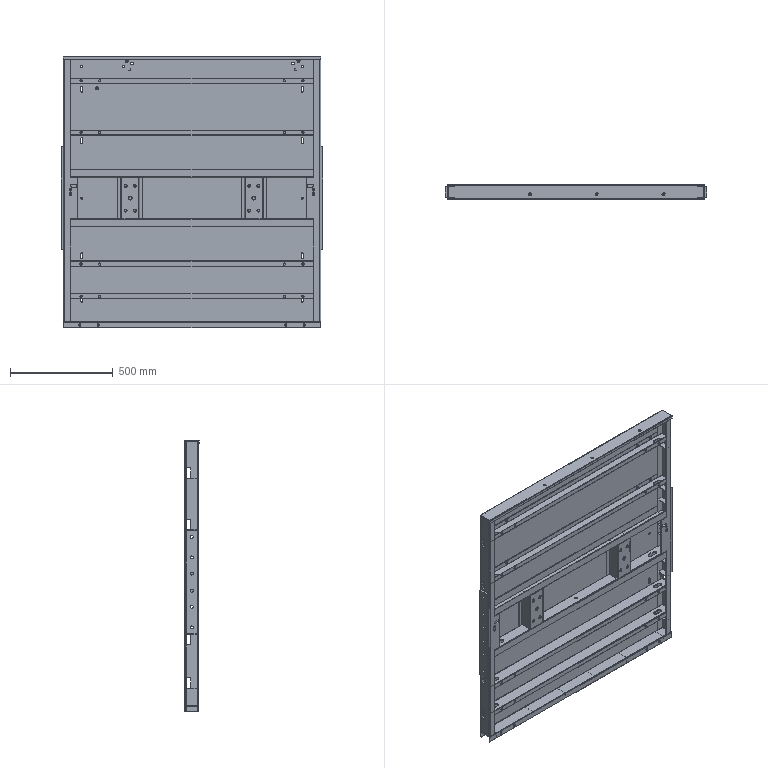Part | 54 solids | 1544 faces | box 1270 x 70 x 1320 mm | volume 10821900 mm3 | plane 960 | cylinder 488 | cone 96 | commonest cylinder face diameters 14.5 x88 10 x78 11 x72 0.4 x36 8.4 x24 20 x24